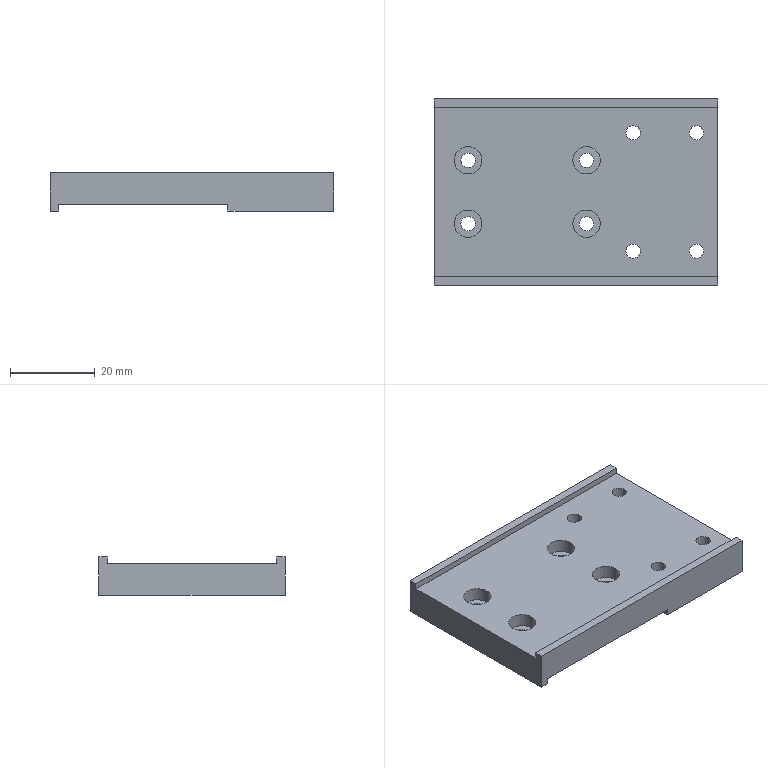Part | STEP file | 11-FG-E00811 | 1 solid | 54 faces | box 67 x 44 x 9 mm | volume 18765 mm3 | cylinder 32 | plane 22 | commonest cylinder face diameters 3.4 x16 6.5 x16